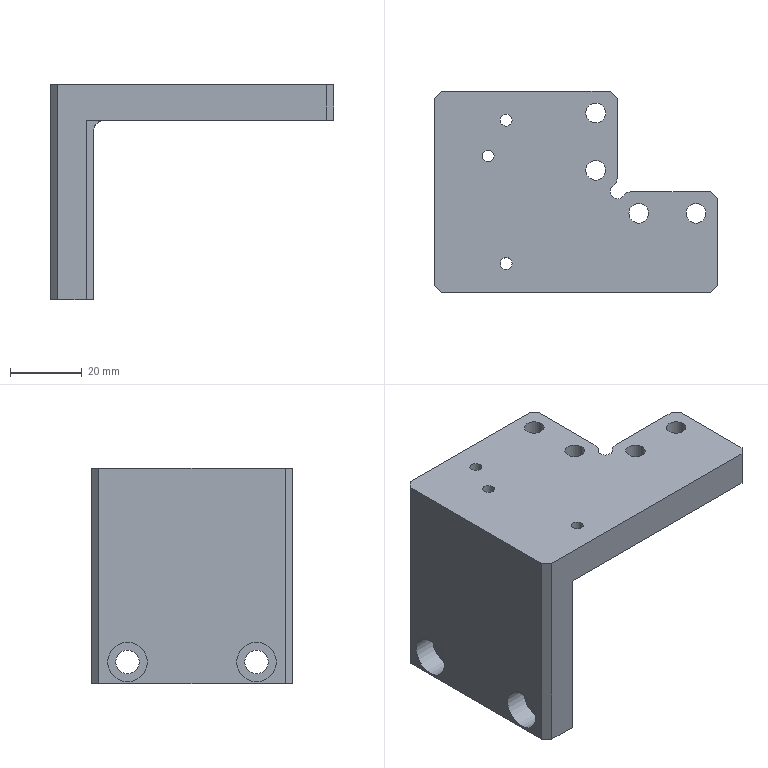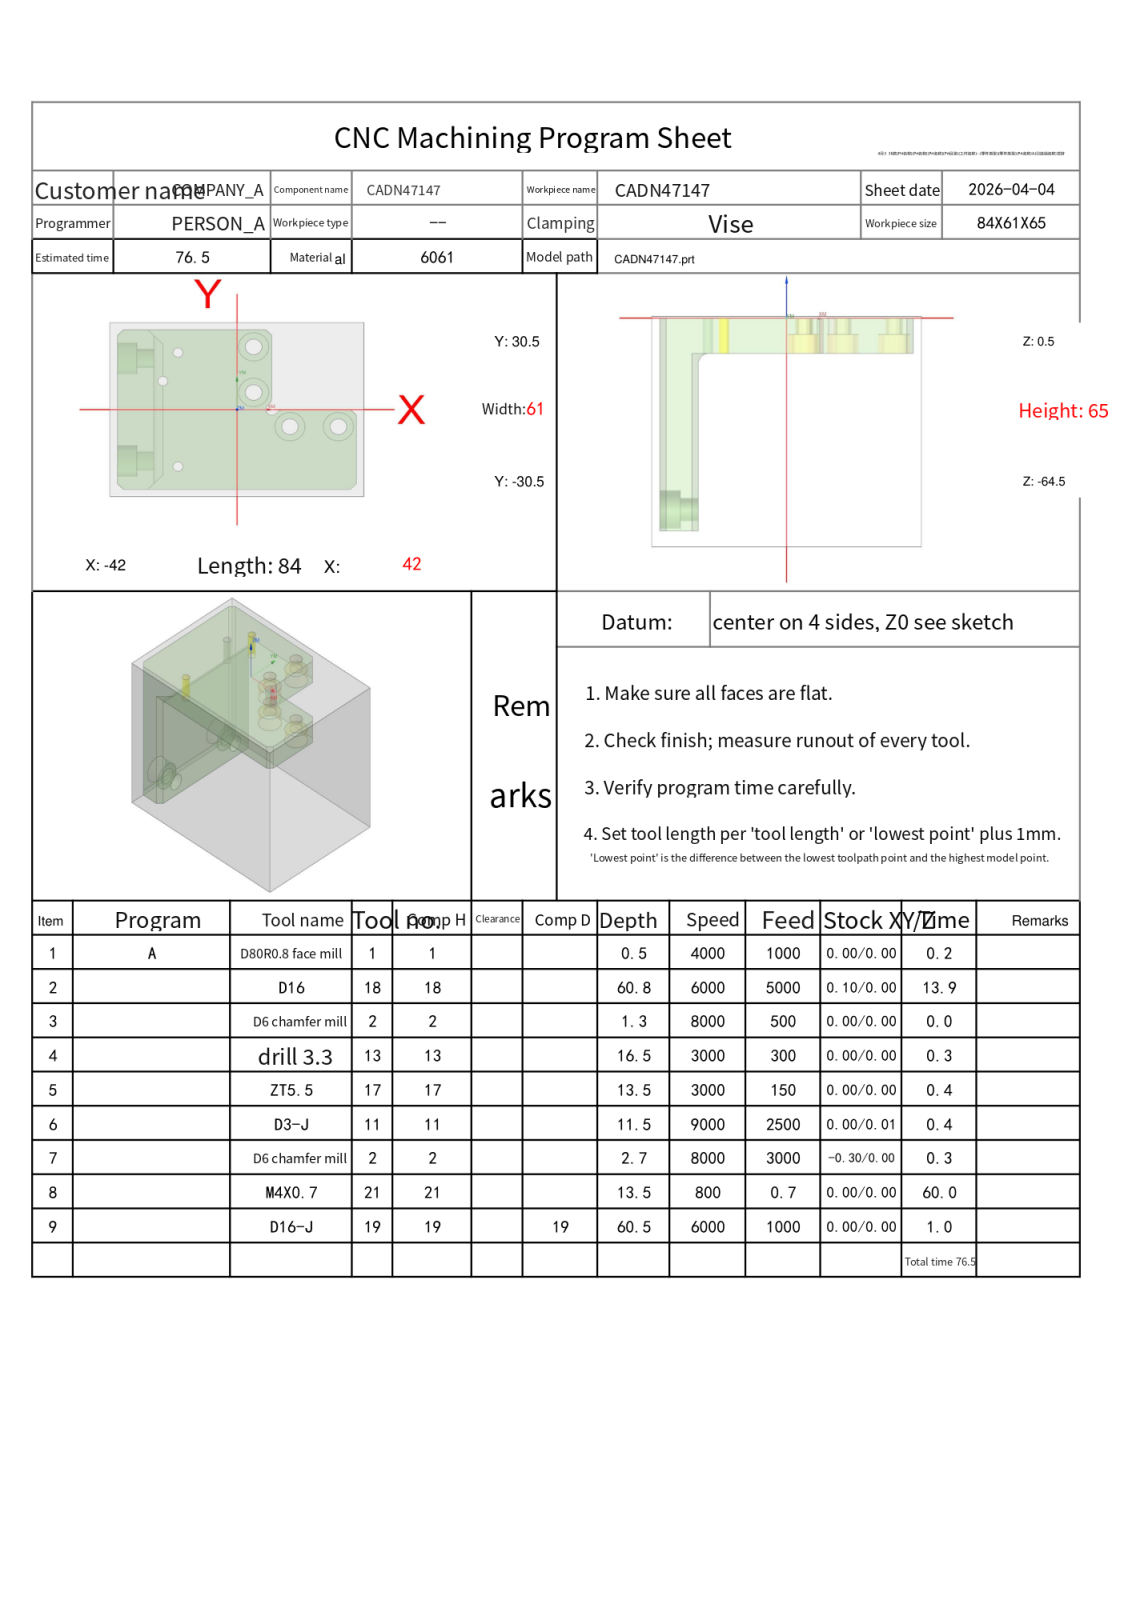NC program | NX | posted by the shop | part box 79 x 56 x 60 mm
Lines 1 to 34 of 9053:
%
O0001
(Machine time: 133.95 MIN)
(===Total Tool:8===)
(T1=D80R0.8 face mill D=80.  R=0.8  D-  H01 Z=0.    )
(T18=D16    D=16.  R=0.   D-  H18 Z=-60.3 )
(T2=D6 chamfer mill   D=6.   R=0.   D-  H02 Z=-2.2  )
(T13=drill 3.3  D=3.3  DR_a=118 D-  H13 Z=-16.  )
(T17=ZT5.5  D=5.5  DR_a=118 D-  H17 Z=-13.  )
(T11=D3-J   D=3.   R=0.   D-  H11 Z=-11.  )
(T21=M4X0.7 D=3.3  DR_a=180 D-  H21 Z=-13.  )
(T19=D16-J  D=16.  R=0.   D19 H19 Z=-60.  )
G80 G90 G17 G49 G40
G91 G28 Z0
M01
N1 T01 M06
(D80R0.8 face mill  D=80. R=0.8 H=01 ce=0.00 di=0.00)
G00 G90 G54 X-84.5 Y0.0 M03 S4000
G43 H01 Z20.
M08
Z2.
G01 Z0.0 F1000.
X-79.5
X79.5
X84.5
Z2.
G00 Z20.
G91 G28 Z0.0
M05
M09
G91 G28 Z0.0
M01